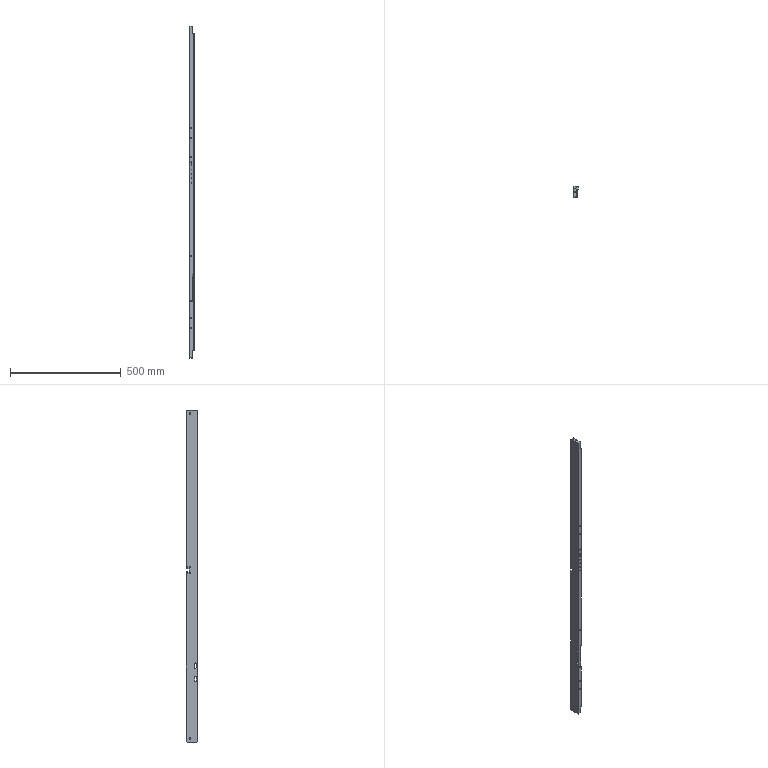Part | SolidWorks | features HoleWzd 7, Cut 3, Chamfer 2, ICE 2, Extrusion 1, Fillet 1 | 1 solid | 125 faces | box 20 x 50 x 1500 mm | volume 1167448 mm3 | cylinder 50 | cone 38 | plane 37 | commonest cylinder face diameters 3.3 x22 5 x16 5.5 x6 6.8 x4 20 x2